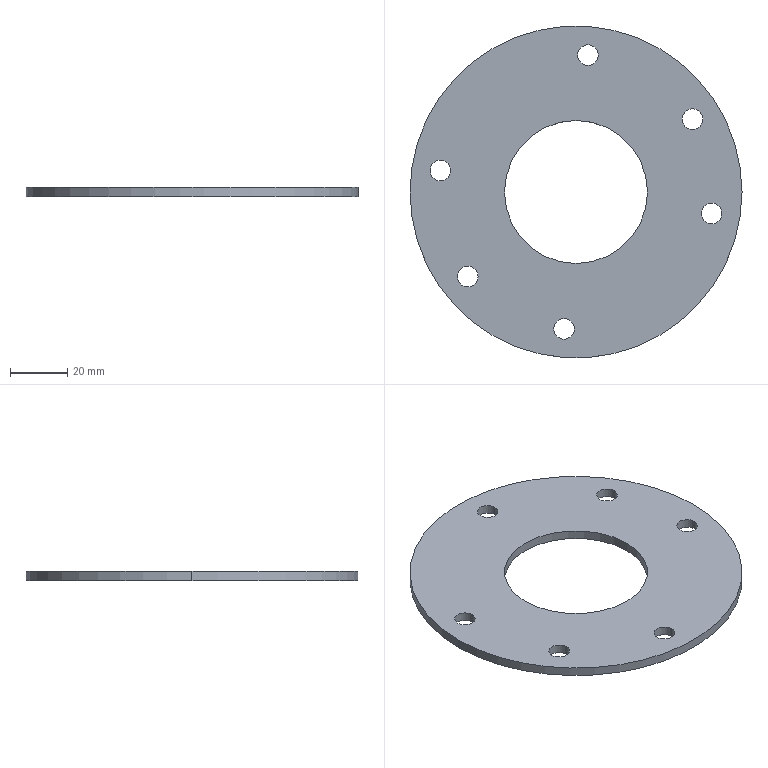Part | SolidWorks | features FlatPattern 1, SMBaseFlange 1, SheetMetal 1 | 1 solid | 18 faces | box 116 x 116 x 3.2 mm | volume 26754 mm3 | cylinder 16 | plane 2 | commonest cylinder face diameters 7.2 x12 50 x2 116 x2
STEP:
#1=CARTESIAN_POINT('',(-7.783,-47.817,-3.2));
#2=VERTEX_POINT('',#1);
#3=CARTESIAN_POINT('',(-0.5835,-47.817,-3.2));
#4=VERTEX_POINT('',#3);
#5=CARTESIAN_POINT('',(-4.183,-47.817,-3.2));
#6=DIRECTION('',(0.,0.,1.));
#7=DIRECTION('',(1.,0.,0.));
#8=AXIS2_PLACEMENT_3D('',#5,#6,#7);
#9=CIRCLE('',#8,3.6);
#10=EDGE_CURVE('',#2,#4,#9,.T.);
#11=ORIENTED_EDGE('',*,*,#10,.F.);
#12=CARTESIAN_POINT('',(-7.783,-47.817,0.));
#13=VERTEX_POINT('',#12);
#14=CARTESIAN_POINT('',(-7.783,-47.817,-3.2));
#15=DIRECTION('',(0.,0.,1.));
#16=VECTOR('',#15,1000.);
#17=LINE('',#14,#16);
#18=EDGE_CURVE('',#2,#13,#17,.T.);
#19=ORIENTED_EDGE('',*,*,#18,.T.);
#20=CARTESIAN_POINT('',(-0.5835,-47.817,0.));
#21=VERTEX_POINT('',#20);
#22=CARTESIAN_POINT('',(-4.183,-47.817,0.));
#23=DIRECTION('',(0.,0.,1.));
#24=DIRECTION('',(1.,0.,0.));
#25=AXIS2_PLACEMENT_3D('',#22,#23,#24);
#26=CIRCLE('',#25,3.6);
#27=EDGE_CURVE('',#13,#21,#26,.T.);
#28=ORIENTED_EDGE('',*,*,#27,.T.);
#29=CARTESIAN_POINT('',(-0.5835,-47.817,-3.2));
#30=DIRECTION('',(0.,0.,1.));
#31=VECTOR('',#30,1000.);
#32=LINE('',#29,#31);
#33=EDGE_CURVE('',#4,#21,#32,.T.);
#34=ORIENTED_EDGE('',*,*,#33,.F.);
#35=EDGE_LOOP('',(#11,#19,#28,#34));
#36=FACE_OUTER_BOUND('',#35,.T.);
#37=CARTESIAN_POINT('',(-4.183,-47.817,-3.2));
#38=DIRECTION('',(0.,0.,1.));
#39=DIRECTION('',(1.,0.,0.));
#40=AXIS2_PLACEMENT_3D('',#37,#38,#39);
#41=CYLINDRICAL_SURFACE('',#40,3.6);
#42=ADVANCED_FACE('',(#36),#41,.F.);
#43=CARTESIAN_POINT('',(-41.425,-29.552,-3.2));
#44=VERTEX_POINT('',#43);
#45=CARTESIAN_POINT('',(-34.225,-29.552,-3.2));
#46=VERTEX_POINT('',#45);
#47=CARTESIAN_POINT('',(-37.825,-29.552,-3.2));
#48=DIRECTION('',(0.,0.,1.));
#49=DIRECTION('',(1.,0.,0.));
#50=AXIS2_PLACEMENT_3D('',#47,#48,#49);
#51=CIRCLE('',#50,3.6);
#52=EDGE_CURVE('',#44,#46,#51,.T.);
#53=ORIENTED_EDGE('',*,*,#52,.F.);
#54=CARTESIAN_POINT('',(-41.425,-29.552,0.));
#55=VERTEX_POINT('',#54);
#56=CARTESIAN_POINT('',(-41.425,-29.552,-3.2));
#57=DIRECTION('',(0.,0.,1.));
#58=VECTOR('',#57,1000.);
#59=LINE('',#56,#58);
#60=EDGE_CURVE('',#44,#55,#59,.T.);
#61=ORIENTED_EDGE('',*,*,#60,.T.);
#62=CARTESIAN_POINT('',(-34.225,-29.552,0.));
#63=VERTEX_POINT('',#62);
#64=CARTESIAN_POINT('',(-37.825,-29.552,0.));
#65=DIRECTION('',(0.,0.,1.));
#66=DIRECTION('',(1.,0.,0.));
#67=AXIS2_PLACEMENT_3D('',#64,#65,#66);
#68=CIRCLE('',#67,3.6);
#69=EDGE_CURVE('',#55,#63,#68,.T.);
#70=ORIENTED_EDGE('',*,*,#69,.T.);
#71=CARTESIAN_POINT('',(-34.225,-29.552,-3.2));
#72=DIRECTION('',(0.,0.,1.));
#73=VECTOR('',#72,1000.);
#74=LINE('',#71,#73);
#75=EDGE_CURVE('',#46,#63,#74,.T.);
#76=ORIENTED_EDGE('',*,*,#75,.F.);
#77=EDGE_LOOP('',(#53,#61,#70,#76));
#78=FACE_OUTER_BOUND('',#77,.T.);
#79=CARTESIAN_POINT('',(-37.825,-29.552,-3.2));
#80=DIRECTION('',(0.,0.,1.));
#81=DIRECTION('',(1.,0.,0.));
#82=AXIS2_PLACEMENT_3D('',#79,#80,#81);
#83=CYLINDRICAL_SURFACE('',#82,3.6);
#84=ADVANCED_FACE('',(#78),#83,.F.);
#85=CARTESIAN_POINT('',(43.809,-7.509,-3.2));
#86=VERTEX_POINT('',#85);
#87=CARTESIAN_POINT('',(51.009,-7.509,-3.2));
#88=VERTEX_POINT('',#87);
#89=CARTESIAN_POINT('',(47.409,-7.509,-3.2));
#90=DIRECTION('',(0.,0.,1.));
#91=DIRECTION('',(1.,0.,0.));
#92=AXIS2_PLACEMENT_3D('',#89,#90,#91);
#93=CIRCLE('',#92,3.6);
#94=EDGE_CURVE('',#86,#88,#93,.T.);
#95=ORIENTED_EDGE('',*,*,#94,.F.);
#96=CARTESIAN_POINT('',(43.809,-7.509,0.));
#97=VERTEX_POINT('',#96);
#98=CARTESIAN_POINT('',(43.809,-7.509,-3.2));
#99=DIRECTION('',(0.,0.,1.));
#100=VECTOR('',#99,1000.);
#101=LINE('',#98,#100);
#102=EDGE_CURVE('',#86,#97,#101,.T.);
#103=ORIENTED_EDGE('',*,*,#102,.T.);
#104=CARTESIAN_POINT('',(51.009,-7.509,0.));
#105=VERTEX_POINT('',#104);
#106=CARTESIAN_POINT('',(47.409,-7.509,0.));
#107=DIRECTION('',(0.,0.,1.));
#108=DIRECTION('',(1.,0.,0.));
#109=AXIS2_PLACEMENT_3D('',#106,#107,#108);
#110=CIRCLE('',#109,3.6);
#111=EDGE_CURVE('',#97,#105,#110,.T.);
#112=ORIENTED_EDGE('',*,*,#111,.T.);
#113=CARTESIAN_POINT('',(51.009,-7.509,-3.2));
#114=DIRECTION('',(0.,0.,1.));
#115=VECTOR('',#114,1000.);
#116=LINE('',#113,#115);
#117=EDGE_CURVE('',#88,#105,#116,.T.);
#118=ORIENTED_EDGE('',*,*,#117,.F.);
#119=EDGE_LOOP('',(#95,#103,#112,#118));
#120=FACE_OUTER_BOUND('',#119,.T.);
#121=CARTESIAN_POINT('',(47.409,-7.509,-3.2));
#122=DIRECTION('',(0.,0.,1.));
#123=DIRECTION('',(1.,0.,0.));
#124=AXIS2_PLACEMENT_3D('',#121,#122,#123);
#125=CYLINDRICAL_SURFACE('',#124,3.6);
#126=ADVANCED_FACE('',(#120),#125,.F.);
#127=CARTESIAN_POINT('',(37.106,25.436,-3.2));
#128=VERTEX_POINT('',#127);
#129=CARTESIAN_POINT('',(44.306,25.436,-3.2));
#130=VERTEX_POINT('',#129);
#131=CARTESIAN_POINT('',(40.706,25.436,-3.2));
#132=DIRECTION('',(0.,0.,1.));
#133=DIRECTION('',(1.,0.,0.));
#134=AXIS2_PLACEMENT_3D('',#131,#132,#133);
#135=CIRCLE('',#134,3.6);
#136=EDGE_CURVE('',#128,#130,#135,.T.);
#137=ORIENTED_EDGE('',*,*,#136,.F.);
#138=CARTESIAN_POINT('',(37.106,25.436,0.));
#139=VERTEX_POINT('',#138);
#140=CARTESIAN_POINT('',(37.106,25.436,-3.2));
#141=DIRECTION('',(0.,0.,1.));
#142=VECTOR('',#141,1000.);
#143=LINE('',#140,#142);
#144=EDGE_CURVE('',#128,#139,#143,.T.);
#145=ORIENTED_EDGE('',*,*,#144,.T.);
#146=CARTESIAN_POINT('',(44.306,25.436,0.));
#147=VERTEX_POINT('',#146);
#148=CARTESIAN_POINT('',(40.706,25.436,0.));
#149=DIRECTION('',(0.,0.,1.));
#150=DIRECTION('',(1.,0.,0.));
#151=AXIS2_PLACEMENT_3D('',#148,#149,#150);
#152=CIRCLE('',#151,3.6);
#153=EDGE_CURVE('',#139,#147,#152,.T.);
#154=ORIENTED_EDGE('',*,*,#153,.T.);
#155=CARTESIAN_POINT('',(44.306,25.436,-3.2));
#156=DIRECTION('',(0.,0.,1.));
#157=VECTOR('',#156,1000.);
#158=LINE('',#155,#157);
#159=EDGE_CURVE('',#130,#147,#158,.T.);
#160=ORIENTED_EDGE('',*,*,#159,.F.);
#161=EDGE_LOOP('',(#137,#145,#154,#160));
#162=FACE_OUTER_BOUND('',#161,.T.);
#163=CARTESIAN_POINT('',(40.706,25.436,-3.2));
#164=DIRECTION('',(0.,0.,1.));
#165=DIRECTION('',(1.,0.,0.));
#166=AXIS2_PLACEMENT_3D('',#163,#164,#165);
#167=CYLINDRICAL_SURFACE('',#166,3.6);
#168=ADVANCED_FACE('',(#162),#167,.F.);
#169=CARTESIAN_POINT('',(0.5835,47.817,-3.2));
#170=VERTEX_POINT('',#169);
#171=CARTESIAN_POINT('',(7.783,47.817,-3.2));
#172=VERTEX_POINT('',#171);
#173=CARTESIAN_POINT('',(4.183,47.817,-3.2));
#174=DIRECTION('',(0.,0.,1.));
#175=DIRECTION('',(1.,0.,0.));
#176=AXIS2_PLACEMENT_3D('',#173,#174,#175);
#177=CIRCLE('',#176,3.6);
#178=EDGE_CURVE('',#170,#172,#177,.T.);
#179=ORIENTED_EDGE('',*,*,#178,.F.);
#180=CARTESIAN_POINT('',(0.5835,47.817,0.));
#181=VERTEX_POINT('',#180);
#182=CARTESIAN_POINT('',(0.5835,47.817,-3.2));
#183=DIRECTION('',(0.,0.,1.));
#184=VECTOR('',#183,1000.);
#185=LINE('',#182,#184);
#186=EDGE_CURVE('',#170,#181,#185,.T.);
#187=ORIENTED_EDGE('',*,*,#186,.T.);
#188=CARTESIAN_POINT('',(7.783,47.817,0.));
#189=VERTEX_POINT('',#188);
#190=CARTESIAN_POINT('',(4.183,47.817,0.));
#191=DIRECTION('',(0.,0.,1.));
#192=DIRECTION('',(1.,0.,0.));
#193=AXIS2_PLACEMENT_3D('',#190,#191,#192);
#194=CIRCLE('',#193,3.6);
#195=EDGE_CURVE('',#181,#189,#194,.T.);
#196=ORIENTED_EDGE('',*,*,#195,.T.);
#197=CARTESIAN_POINT('',(7.783,47.817,-3.2));
#198=DIRECTION('',(0.,0.,1.));
#199=VECTOR('',#198,1000.);
#200=LINE('',#197,#199);
#201=EDGE_CURVE('',#172,#189,#200,.T.);
#202=ORIENTED_EDGE('',*,*,#201,.F.);
#203=EDGE_LOOP('',(#179,#187,#196,#202));
#204=FACE_OUTER_BOUND('',#203,.T.);
#205=CARTESIAN_POINT('',(4.183,47.817,-3.2));
#206=DIRECTION('',(0.,0.,1.));
#207=DIRECTION('',(1.,0.,0.));
#208=AXIS2_PLACEMENT_3D('',#205,#206,#207);
#209=CYLINDRICAL_SURFACE('',#208,3.6);
#210=ADVANCED_FACE('',(#204),#209,.F.);
#211=CARTESIAN_POINT('',(-51.009,7.509,-3.2));
#212=VERTEX_POINT('',#211);
#213=CARTESIAN_POINT('',(-43.809,7.509,-3.2));
#214=VERTEX_POINT('',#213);
#215=CARTESIAN_POINT('',(-47.409,7.509,-3.2));
#216=DIRECTION('',(0.,0.,1.));
#217=DIRECTION('',(1.,0.,0.));
#218=AXIS2_PLACEMENT_3D('',#215,#216,#217);
#219=CIRCLE('',#218,3.6);
#220=EDGE_CURVE('',#212,#214,#219,.T.);
#221=ORIENTED_EDGE('',*,*,#220,.F.);
#222=CARTESIAN_POINT('',(-51.009,7.509,0.));
#223=VERTEX_POINT('',#222);
#224=CARTESIAN_POINT('',(-51.009,7.509,-3.2));
#225=DIRECTION('',(0.,0.,1.));
#226=VECTOR('',#225,1000.);
#227=LINE('',#224,#226);
#228=EDGE_CURVE('',#212,#223,#227,.T.);
#229=ORIENTED_EDGE('',*,*,#228,.T.);
#230=CARTESIAN_POINT('',(-43.809,7.509,0.));
#231=VERTEX_POINT('',#230);
#232=CARTESIAN_POINT('',(-47.409,7.509,0.));
#233=DIRECTION('',(0.,0.,1.));
#234=DIRECTION('',(1.,0.,0.));
#235=AXIS2_PLACEMENT_3D('',#232,#233,#234);
#236=CIRCLE('',#235,3.6);
#237=EDGE_CURVE('',#223,#231,#236,.T.);
#238=ORIENTED_EDGE('',*,*,#237,.T.);
#239=CARTESIAN_POINT('',(-43.809,7.509,-3.2));
#240=DIRECTION('',(0.,0.,1.));
#241=VECTOR('',#240,1000.);
#242=LINE('',#239,#241);
#243=EDGE_CURVE('',#214,#231,#242,.T.);
#244=ORIENTED_EDGE('',*,*,#243,.F.);
#245=EDGE_LOOP('',(#221,#229,#238,#244));
#246=FACE_OUTER_BOUND('',#245,.T.);
#247=CARTESIAN_POINT('',(-47.409,7.509,-3.2));
#248=DIRECTION('',(0.,0.,1.));
#249=DIRECTION('',(1.,0.,0.));
#250=AXIS2_PLACEMENT_3D('',#247,#248,#249);
#251=CYLINDRICAL_SURFACE('',#250,3.6);
#252=ADVANCED_FACE('',(#246),#251,.F.);
#253=CARTESIAN_POINT('',(-25.,0.,-3.2));
#254=VERTEX_POINT('',#253);
#255=CARTESIAN_POINT('',(25.,0.,-3.2));
#256=VERTEX_POINT('',#255);
#257=CARTESIAN_POINT('',(0.,0.,-3.2));
#258=DIRECTION('',(0.,0.,1.));
#259=DIRECTION('',(1.,0.,0.));
#260=AXIS2_PLACEMENT_3D('',#257,#258,#259);
#261=CIRCLE('',#260,25.);
#262=EDGE_CURVE('',#254,#256,#261,.T.);
#263=ORIENTED_EDGE('',*,*,#262,.F.);
#264=CARTESIAN_POINT('',(-25.,0.,0.));
#265=VERTEX_POINT('',#264);
#266=CARTESIAN_POINT('',(-25.,0.,-3.2));
#267=DIRECTION('',(0.,0.,1.));
#268=VECTOR('',#267,1000.);
#269=LINE('',#266,#268);
#270=EDGE_CURVE('',#254,#265,#269,.T.);
#271=ORIENTED_EDGE('',*,*,#270,.T.);
#272=CARTESIAN_POINT('',(25.,0.,0.));
#273=VERTEX_POINT('',#272);
#274=CARTESIAN_POINT('',(0.,0.,0.));
#275=DIRECTION('',(0.,0.,1.));
#276=DIRECTION('',(1.,0.,0.));
#277=AXIS2_PLACEMENT_3D('',#274,#275,#276);
#278=CIRCLE('',#277,25.);
#279=EDGE_CURVE('',#265,#273,#278,.T.);
#280=ORIENTED_EDGE('',*,*,#279,.T.);
#281=CARTESIAN_POINT('',(25.,0.,-3.2));
#282=DIRECTION('',(0.,0.,1.));
#283=VECTOR('',#282,1000.);
#284=LINE('',#281,#283);
#285=EDGE_CURVE('',#256,#273,#284,.T.);
#286=ORIENTED_EDGE('',*,*,#285,.F.);
#287=EDGE_LOOP('',(#263,#271,#280,#286));
#288=FACE_OUTER_BOUND('',#287,.T.);
#289=CARTESIAN_POINT('',(0.,0.,-3.2));
#290=DIRECTION('',(0.,0.,1.));
#291=DIRECTION('',(1.,0.,0.));
#292=AXIS2_PLACEMENT_3D('',#289,#290,#291);
#293=CYLINDRICAL_SURFACE('',#292,25.);
#294=ADVANCED_FACE('',(#288),#293,.F.);
#295=CARTESIAN_POINT('',(58.,0.,-3.2));
#296=VERTEX_POINT('',#295);
#297=CARTESIAN_POINT('',(-58.,0.,-3.2));
#298=VERTEX_POINT('',#297);
#299=CARTESIAN_POINT('',(0.,0.,-3.2));
#300=DIRECTION('',(0.,0.,1.));
#301=DIRECTION('',(1.,0.,0.));
#302=AXIS2_PLACEMENT_3D('',#299,#300,#301);
#303=CIRCLE('',#302,58.);
#304=EDGE_CURVE('',#296,#298,#303,.T.);
#305=ORIENTED_EDGE('',*,*,#304,.T.);
#306=CARTESIAN_POINT('',(-58.,0.,0.));
#307=VERTEX_POINT('',#306);
#308=CARTESIAN_POINT('',(-58.,0.,-3.2));
#309=DIRECTION('',(0.,0.,1.));
#310=VECTOR('',#309,1000.);
#311=LINE('',#308,#310);
#312=EDGE_CURVE('',#298,#307,#311,.T.);
#313=ORIENTED_EDGE('',*,*,#312,.T.);
#314=CARTESIAN_POINT('',(58.,0.,0.));
#315=VERTEX_POINT('',#314);
#316=CARTESIAN_POINT('',(0.,0.,0.));
#317=DIRECTION('',(0.,0.,1.));
#318=DIRECTION('',(1.,0.,0.));
#319=AXIS2_PLACEMENT_3D('',#316,#317,#318);
#320=CIRCLE('',#319,58.);
#321=EDGE_CURVE('',#315,#307,#320,.T.);
#322=ORIENTED_EDGE('',*,*,#321,.F.);
#323=CARTESIAN_POINT('',(58.,0.,-3.2));
#324=DIRECTION('',(0.,0.,1.));
#325=VECTOR('',#324,1000.);
#326=LINE('',#323,#325);
#327=EDGE_CURVE('',#296,#315,#326,.T.);
#328=ORIENTED_EDGE('',*,*,#327,.F.);
#329=EDGE_LOOP('',(#305,#313,#322,#328));
#330=FACE_OUTER_BOUND('',#329,.T.);
#331=CARTESIAN_POINT('',(0.,0.,-3.2));
#332=DIRECTION('',(0.,0.,1.));
#333=DIRECTION('',(1.,0.,0.));
#334=AXIS2_PLACEMENT_3D('',#331,#332,#333);
#335=CYLINDRICAL_SURFACE('',#334,58.);
#336=ADVANCED_FACE('',(#330),#335,.T.);
#337=ORIENTED_EDGE('',*,*,#312,.F.);
#338=CARTESIAN_POINT('',(0.,0.,-3.2));
#339=DIRECTION('',(0.,0.,1.));
#340=DIRECTION('',(1.,0.,0.));
#341=AXIS2_PLACEMENT_3D('',#338,#339,#340);
#342=CIRCLE('',#341,58.);
#343=EDGE_CURVE('',#298,#296,#342,.T.);
#344=ORIENTED_EDGE('',*,*,#343,.T.);
#345=ORIENTED_EDGE('',*,*,#327,.T.);
#346=CARTESIAN_POINT('',(0.,0.,0.));
#347=DIRECTION('',(0.,0.,1.));
#348=DIRECTION('',(1.,0.,0.));
#349=AXIS2_PLACEMENT_3D('',#346,#347,#348);
#350=CIRCLE('',#349,58.);
#351=EDGE_CURVE('',#307,#315,#350,.T.);
#352=ORIENTED_EDGE('',*,*,#351,.F.);
#353=EDGE_LOOP('',(#337,#344,#345,#352));
#354=FACE_OUTER_BOUND('',#353,.T.);
#355=CARTESIAN_POINT('',(0.,0.,-3.2));
#356=DIRECTION('',(0.,0.,1.));
#357=DIRECTION('',(1.,0.,0.));
#358=AXIS2_PLACEMENT_3D('',#355,#356,#357);
#359=CYLINDRICAL_SURFACE('',#358,58.);
#360=ADVANCED_FACE('',(#354),#359,.T.);
#361=CARTESIAN_POINT('',(-4.183,-47.817,-3.2));
#362=DIRECTION('',(0.,0.,1.));
#363=DIRECTION('',(1.,0.,0.));
#364=AXIS2_PLACEMENT_3D('',#361,#362,#363);
#365=CIRCLE('',#364,3.6);
#366=EDGE_CURVE('',#4,#2,#365,.T.);
#367=ORIENTED_EDGE('',*,*,#366,.T.);
#368=ORIENTED_EDGE('',*,*,#10,.T.);
#369=EDGE_LOOP('',(#367,#368));
#370=FACE_BOUND('',#369,.T.);
#371=CARTESIAN_POINT('',(-37.825,-29.552,-3.2));
#372=DIRECTION('',(0.,0.,1.));
#373=DIRECTION('',(1.,0.,0.));
#374=AXIS2_PLACEMENT_3D('',#371,#372,#373);
#375=CIRCLE('',#374,3.6);
#376=EDGE_CURVE('',#46,#44,#375,.T.);
#377=ORIENTED_EDGE('',*,*,#376,.T.);
#378=ORIENTED_EDGE('',*,*,#52,.T.);
#379=EDGE_LOOP('',(#377,#378));
#380=FACE_BOUND('',#379,.T.);
#381=CARTESIAN_POINT('',(47.409,-7.509,-3.2));
#382=DIRECTION('',(0.,0.,1.));
#383=DIRECTION('',(1.,0.,0.));
#384=AXIS2_PLACEMENT_3D('',#381,#382,#383);
#385=CIRCLE('',#384,3.6);
#386=EDGE_CURVE('',#88,#86,#385,.T.);
#387=ORIENTED_EDGE('',*,*,#386,.T.);
#388=ORIENTED_EDGE('',*,*,#94,.T.);
#389=EDGE_LOOP('',(#387,#388));
#390=FACE_BOUND('',#389,.T.);
#391=CARTESIAN_POINT('',(40.706,25.436,-3.2));
#392=DIRECTION('',(0.,0.,1.));
#393=DIRECTION('',(1.,0.,0.));
#394=AXIS2_PLACEMENT_3D('',#391,#392,#393);
#395=CIRCLE('',#394,3.6);
#396=EDGE_CURVE('',#130,#128,#395,.T.);
#397=ORIENTED_EDGE('',*,*,#396,.T.);
#398=ORIENTED_EDGE('',*,*,#136,.T.);
#399=EDGE_LOOP('',(#397,#398));
#400=FACE_BOUND('',#399,.T.);
#401=CARTESIAN_POINT('',(4.183,47.817,-3.2));
#402=DIRECTION('',(0.,0.,1.));
#403=DIRECTION('',(1.,0.,0.));
#404=AXIS2_PLACEMENT_3D('',#401,#402,#403);
#405=CIRCLE('',#404,3.6);
#406=EDGE_CURVE('',#172,#170,#405,.T.);
#407=ORIENTED_EDGE('',*,*,#406,.T.);
#408=ORIENTED_EDGE('',*,*,#178,.T.);
#409=EDGE_LOOP('',(#407,#408));
#410=FACE_BOUND('',#409,.T.);
#411=CARTESIAN_POINT('',(-47.409,7.509,-3.2));
#412=DIRECTION('',(0.,0.,1.));
#413=DIRECTION('',(1.,0.,0.));
#414=AXIS2_PLACEMENT_3D('',#411,#412,#413);
#415=CIRCLE('',#414,3.6);
#416=EDGE_CURVE('',#214,#212,#415,.T.);
#417=ORIENTED_EDGE('',*,*,#416,.T.);
#418=ORIENTED_EDGE('',*,*,#220,.T.);
#419=EDGE_LOOP('',(#417,#418));
#420=FACE_BOUND('',#419,.T.);
#421=CARTESIAN_POINT('',(0.,0.,-3.2));
#422=DIRECTION('',(0.,0.,1.));
#423=DIRECTION('',(1.,0.,0.));
#424=AXIS2_PLACEMENT_3D('',#421,#422,#423);
#425=CIRCLE('',#424,25.);
#426=EDGE_CURVE('',#256,#254,#425,.T.);
#427=ORIENTED_EDGE('',*,*,#426,.T.);
#428=ORIENTED_EDGE('',*,*,#262,.T.);
#429=EDGE_LOOP('',(#427,#428));
#430=FACE_BOUND('',#429,.T.);
#431=ORIENTED_EDGE('',*,*,#304,.F.);
#432=ORIENTED_EDGE('',*,*,#343,.F.);
#433=EDGE_LOOP('',(#431,#432));
#434=FACE_OUTER_BOUND('',#433,.T.);
#435=CARTESIAN_POINT('',(0.,0.,-3.2));
#436=DIRECTION('',(0.,0.,1.));
#437=DIRECTION('',(1.,0.,0.));
#438=AXIS2_PLACEMENT_3D('',#435,#436,#437);
#439=PLANE('',#438);
#440=ADVANCED_FACE('',(#370,#380,#390,#400,#410,#420,#430,#434),#439,.F.);
#441=CARTESIAN_POINT('',(-4.183,-47.817,0.));
#442=DIRECTION('',(0.,0.,1.));
#443=DIRECTION('',(1.,0.,0.));
#444=AXIS2_PLACEMENT_3D('',#441,#442,#443);
#445=CIRCLE('',#444,3.6);
#446=EDGE_CURVE('',#21,#13,#445,.T.);
#447=ORIENTED_EDGE('',*,*,#446,.F.);
#448=ORIENTED_EDGE('',*,*,#27,.F.);
#449=EDGE_LOOP('',(#447,#448));
#450=FACE_BOUND('',#449,.T.);
#451=CARTESIAN_POINT('',(-37.825,-29.552,0.));
#452=DIRECTION('',(0.,0.,1.));
#453=DIRECTION('',(1.,0.,0.));
#454=AXIS2_PLACEMENT_3D('',#451,#452,#453);
#455=CIRCLE('',#454,3.6);
#456=EDGE_CURVE('',#63,#55,#455,.T.);
#457=ORIENTED_EDGE('',*,*,#456,.F.);
#458=ORIENTED_EDGE('',*,*,#69,.F.);
#459=EDGE_LOOP('',(#457,#458));
#460=FACE_BOUND('',#459,.T.);
#461=CARTESIAN_POINT('',(47.409,-7.509,0.));
#462=DIRECTION('',(0.,0.,1.));
#463=DIRECTION('',(1.,0.,0.));
#464=AXIS2_PLACEMENT_3D('',#461,#462,#463);
#465=CIRCLE('',#464,3.6);
#466=EDGE_CURVE('',#105,#97,#465,.T.);
#467=ORIENTED_EDGE('',*,*,#466,.F.);
#468=ORIENTED_EDGE('',*,*,#111,.F.);
#469=EDGE_LOOP('',(#467,#468));
#470=FACE_BOUND('',#469,.T.);
#471=CARTESIAN_POINT('',(40.706,25.436,0.));
#472=DIRECTION('',(0.,0.,1.));
#473=DIRECTION('',(1.,0.,0.));
#474=AXIS2_PLACEMENT_3D('',#471,#472,#473);
#475=CIRCLE('',#474,3.6);
#476=EDGE_CURVE('',#147,#139,#475,.T.);
#477=ORIENTED_EDGE('',*,*,#476,.F.);
#478=ORIENTED_EDGE('',*,*,#153,.F.);
#479=EDGE_LOOP('',(#477,#478));
#480=FACE_BOUND('',#479,.T.);
#481=CARTESIAN_POINT('',(4.183,47.817,0.));
#482=DIRECTION('',(0.,0.,1.));
#483=DIRECTION('',(1.,0.,0.));
#484=AXIS2_PLACEMENT_3D('',#481,#482,#483);
#485=CIRCLE('',#484,3.6);
#486=EDGE_CURVE('',#189,#181,#485,.T.);
#487=ORIENTED_EDGE('',*,*,#486,.F.);
#488=ORIENTED_EDGE('',*,*,#195,.F.);
#489=EDGE_LOOP('',(#487,#488));
#490=FACE_BOUND('',#489,.T.);
#491=CARTESIAN_POINT('',(-47.409,7.509,0.));
#492=DIRECTION('',(0.,0.,1.));
#493=DIRECTION('',(1.,0.,0.));
#494=AXIS2_PLACEMENT_3D('',#491,#492,#493);
#495=CIRCLE('',#494,3.6);
#496=EDGE_CURVE('',#231,#223,#495,.T.);
#497=ORIENTED_EDGE('',*,*,#496,.F.);
#498=ORIENTED_EDGE('',*,*,#237,.F.);
#499=EDGE_LOOP('',(#497,#498));
#500=FACE_BOUND('',#499,.T.);
#501=CARTESIAN_POINT('',(0.,0.,0.));
#502=DIRECTION('',(0.,0.,1.));
#503=DIRECTION('',(1.,0.,0.));
#504=AXIS2_PLACEMENT_3D('',#501,#502,#503);
#505=CIRCLE('',#504,25.);
#506=EDGE_CURVE('',#273,#265,#505,.T.);
#507=ORIENTED_EDGE('',*,*,#506,.F.);
#508=ORIENTED_EDGE('',*,*,#279,.F.);
#509=EDGE_LOOP('',(#507,#508));
#510=FACE_BOUND('',#509,.T.);
#511=ORIENTED_EDGE('',*,*,#321,.T.);
#512=ORIENTED_EDGE('',*,*,#351,.T.);
#513=EDGE_LOOP('',(#511,#512));
#514=FACE_OUTER_BOUND('',#513,.T.);
#515=CARTESIAN_POINT('',(0.,0.,0.));
#516=DIRECTION('',(0.,0.,1.));
#517=DIRECTION('',(1.,0.,0.));
#518=AXIS2_PLACEMENT_3D('',#515,#516,#517);
#519=PLANE('',#518);
#520=ADVANCED_FACE('',(#450,#460,#470,#480,#490,#500,#510,#514),#519,.T.);
#521=ORIENTED_EDGE('',*,*,#270,.F.);
#522=ORIENTED_EDGE('',*,*,#426,.F.);
#523=ORIENTED_EDGE('',*,*,#285,.T.);
#524=ORIENTED_EDGE('',*,*,#506,.T.);
#525=EDGE_LOOP('',(#521,#522,#523,#524));
#526=FACE_OUTER_BOUND('',#525,.T.);
#527=CARTESIAN_POINT('',(0.,0.,-3.2));
#528=DIRECTION('',(0.,0.,1.));
#529=DIRECTION('',(1.,0.,0.));
#530=AXIS2_PLACEMENT_3D('',#527,#528,#529);
#531=CYLINDRICAL_SURFACE('',#530,25.);
#532=ADVANCED_FACE('',(#526),#531,.F.);
#533=ORIENTED_EDGE('',*,*,#228,.F.);
#534=ORIENTED_EDGE('',*,*,#416,.F.);
#535=ORIENTED_EDGE('',*,*,#243,.T.);
#536=ORIENTED_EDGE('',*,*,#496,.T.);
#537=EDGE_LOOP('',(#533,#534,#535,#536));
#538=FACE_OUTER_BOUND('',#537,.T.);
#539=CARTESIAN_POINT('',(-47.409,7.509,-3.2));
#540=DIRECTION('',(0.,0.,1.));
#541=DIRECTION('',(1.,0.,0.));
#542=AXIS2_PLACEMENT_3D('',#539,#540,#541);
#543=CYLINDRICAL_SURFACE('',#542,3.6);
#544=ADVANCED_FACE('',(#538),#543,.F.);
#545=ORIENTED_EDGE('',*,*,#186,.F.);
#546=ORIENTED_EDGE('',*,*,#406,.F.);
#547=ORIENTED_EDGE('',*,*,#201,.T.);
#548=ORIENTED_EDGE('',*,*,#486,.T.);
#549=EDGE_LOOP('',(#545,#546,#547,#548));
#550=FACE_OUTER_BOUND('',#549,.T.);
#551=CARTESIAN_POINT('',(4.183,47.817,-3.2));
#552=DIRECTION('',(0.,0.,1.));
#553=DIRECTION('',(1.,0.,0.));
#554=AXIS2_PLACEMENT_3D('',#551,#552,#553);
#555=CYLINDRICAL_SURFACE('',#554,3.6);
#556=ADVANCED_FACE('',(#550),#555,.F.);
#557=ORIENTED_EDGE('',*,*,#144,.F.);
#558=ORIENTED_EDGE('',*,*,#396,.F.);
#559=ORIENTED_EDGE('',*,*,#159,.T.);
#560=ORIENTED_EDGE('',*,*,#476,.T.);
#561=EDGE_LOOP('',(#557,#558,#559,#560));
#562=FACE_OUTER_BOUND('',#561,.T.);
#563=CARTESIAN_POINT('',(40.706,25.436,-3.2));
#564=DIRECTION('',(0.,0.,1.));
#565=DIRECTION('',(1.,0.,0.));
#566=AXIS2_PLACEMENT_3D('',#563,#564,#565);
#567=CYLINDRICAL_SURFACE('',#566,3.6);
#568=ADVANCED_FACE('',(#562),#567,.F.);
#569=ORIENTED_EDGE('',*,*,#102,.F.);
#570=ORIENTED_EDGE('',*,*,#386,.F.);
#571=ORIENTED_EDGE('',*,*,#117,.T.);
#572=ORIENTED_EDGE('',*,*,#466,.T.);
#573=EDGE_LOOP('',(#569,#570,#571,#572));
#574=FACE_OUTER_BOUND('',#573,.T.);
#575=CARTESIAN_POINT('',(47.409,-7.509,-3.2));
#576=DIRECTION('',(0.,0.,1.));
#577=DIRECTION('',(1.,0.,0.));
#578=AXIS2_PLACEMENT_3D('',#575,#576,#577);
#579=CYLINDRICAL_SURFACE('',#578,3.6);
#580=ADVANCED_FACE('',(#574),#579,.F.);
#581=ORIENTED_EDGE('',*,*,#60,.F.);
#582=ORIENTED_EDGE('',*,*,#376,.F.);
#583=ORIENTED_EDGE('',*,*,#75,.T.);
#584=ORIENTED_EDGE('',*,*,#456,.T.);
#585=EDGE_LOOP('',(#581,#582,#583,#584));
#586=FACE_OUTER_BOUND('',#585,.T.);
#587=CARTESIAN_POINT('',(-37.825,-29.552,-3.2));
#588=DIRECTION('',(0.,0.,1.));
#589=DIRECTION('',(1.,0.,0.));
#590=AXIS2_PLACEMENT_3D('',#587,#588,#589);
#591=CYLINDRICAL_SURFACE('',#590,3.6);
#592=ADVANCED_FACE('',(#586),#591,.F.);
#593=ORIENTED_EDGE('',*,*,#18,.F.);
#594=ORIENTED_EDGE('',*,*,#366,.F.);
#595=ORIENTED_EDGE('',*,*,#33,.T.);
#596=ORIENTED_EDGE('',*,*,#446,.T.);
#597=EDGE_LOOP('',(#593,#594,#595,#596));
#598=FACE_OUTER_BOUND('',#597,.T.);
#599=CARTESIAN_POINT('',(-4.183,-47.817,-3.2));
#600=DIRECTION('',(0.,0.,1.));
#601=DIRECTION('',(1.,0.,0.));
#602=AXIS2_PLACEMENT_3D('',#599,#600,#601);
#603=CYLINDRICAL_SURFACE('',#602,3.6);
#604=ADVANCED_FACE('',(#598),#603,.F.);
#605=CLOSED_SHELL('',(#42,#84,#126,#168,#210,#252,#294,#336,#360,#440,#520,#532,#544,#556,#568,#580,#592,#604));
#606=MANIFOLD_SOLID_BREP('',#605);
#607=CARTESIAN_POINT('',(0.,0.,0.));
#608=DIRECTION('',(0.,0.,1.));
#609=DIRECTION('',(1.,0.,0.));
#610=AXIS2_PLACEMENT_3D('',#607,#608,#609);
#611=(LENGTH_UNIT()NAMED_UNIT(*)SI_UNIT(.MILLI.,.METRE.));
#612=UNCERTAINTY_MEASURE_WITH_UNIT(LENGTH_MEASURE(0.00001),#611,'','');
#613=(NAMED_UNIT(*)PLANE_ANGLE_UNIT()SI_UNIT($,.RADIAN.));
#614=(NAMED_UNIT(*)SI_UNIT($,.STERADIAN.)SOLID_ANGLE_UNIT());
#615=(GEOMETRIC_REPRESENTATION_CONTEXT(3)GLOBAL_UNCERTAINTY_ASSIGNED_CONTEXT((#612))GLOBAL_UNIT_ASSIGNED_CONTEXT((#611,#613,#614))REPRESENTATION_CONTEXT('',''));
#616=ADVANCED_BREP_SHAPE_REPRESENTATION('',(#606,#610),#615);